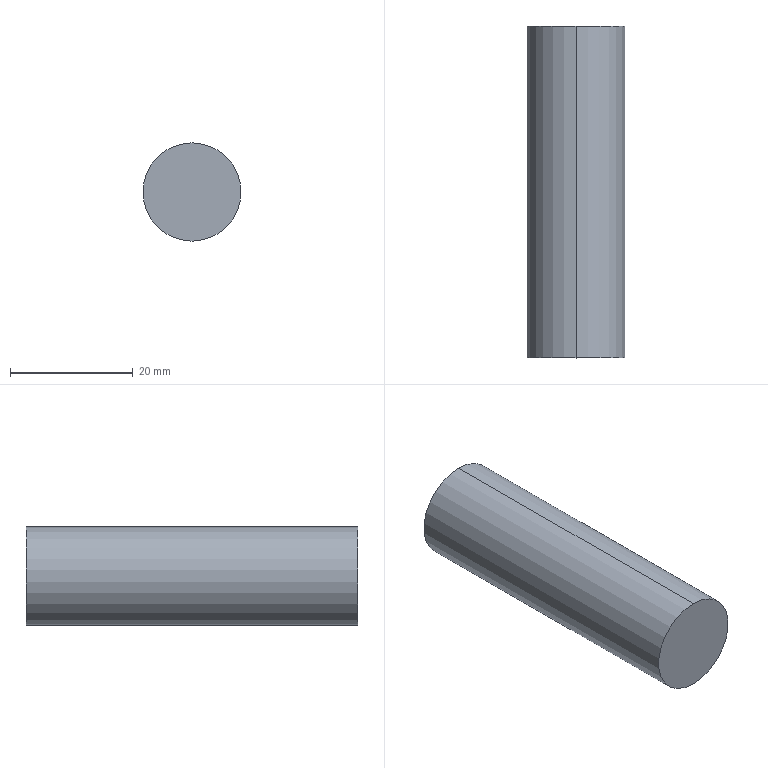Part | SolidWorks | features Extrusion 1 | 1 solid | 4 faces | box 16 x 54 x 16 mm | volume 10857 mm3 | cylinder 2 | plane 2 | commonest cylinder face diameters 16 x2
STEP:
#1=CARTESIAN_POINT('',(0.,54.,8.));
#2=VERTEX_POINT('',#1);
#3=CARTESIAN_POINT('',(0.,54.,-8.));
#4=VERTEX_POINT('',#3);
#5=CARTESIAN_POINT('',(0.,54.,0.));
#6=DIRECTION('',(0.,1.,0.));
#7=DIRECTION('',(0.,0.,1.));
#8=AXIS2_PLACEMENT_3D('',#5,#6,#7);
#9=CIRCLE('',#8,8.);
#10=EDGE_CURVE('',#2,#4,#9,.T.);
#11=ORIENTED_EDGE('',*,*,#10,.F.);
#12=CARTESIAN_POINT('',(0.,0.,8.));
#13=VERTEX_POINT('',#12);
#14=CARTESIAN_POINT('',(0.,54.,8.));
#15=DIRECTION('',(0.,-1.,0.));
#16=VECTOR('',#15,1000.);
#17=LINE('',#14,#16);
#18=EDGE_CURVE('',#2,#13,#17,.T.);
#19=ORIENTED_EDGE('',*,*,#18,.T.);
#20=CARTESIAN_POINT('',(0.,0.,-8.));
#21=VERTEX_POINT('',#20);
#22=CARTESIAN_POINT('',(0.,0.,0.));
#23=DIRECTION('',(0.,1.,0.));
#24=DIRECTION('',(0.,0.,1.));
#25=AXIS2_PLACEMENT_3D('',#22,#23,#24);
#26=CIRCLE('',#25,8.);
#27=EDGE_CURVE('',#13,#21,#26,.T.);
#28=ORIENTED_EDGE('',*,*,#27,.T.);
#29=CARTESIAN_POINT('',(0.,54.,-8.));
#30=DIRECTION('',(0.,-1.,0.));
#31=VECTOR('',#30,1000.);
#32=LINE('',#29,#31);
#33=EDGE_CURVE('',#4,#21,#32,.T.);
#34=ORIENTED_EDGE('',*,*,#33,.F.);
#35=EDGE_LOOP('',(#11,#19,#28,#34));
#36=FACE_OUTER_BOUND('',#35,.T.);
#37=CARTESIAN_POINT('',(0.,54.,0.));
#38=DIRECTION('',(0.,-1.,0.));
#39=DIRECTION('',(0.,0.,-1.));
#40=AXIS2_PLACEMENT_3D('',#37,#38,#39);
#41=CYLINDRICAL_SURFACE('',#40,8.);
#42=ADVANCED_FACE('',(#36),#41,.T.);
#43=ORIENTED_EDGE('',*,*,#18,.F.);
#44=CARTESIAN_POINT('',(0.,54.,0.));
#45=DIRECTION('',(0.,1.,0.));
#46=DIRECTION('',(0.,0.,1.));
#47=AXIS2_PLACEMENT_3D('',#44,#45,#46);
#48=CIRCLE('',#47,8.);
#49=EDGE_CURVE('',#4,#2,#48,.T.);
#50=ORIENTED_EDGE('',*,*,#49,.F.);
#51=ORIENTED_EDGE('',*,*,#33,.T.);
#52=CARTESIAN_POINT('',(0.,0.,0.));
#53=DIRECTION('',(0.,1.,0.));
#54=DIRECTION('',(0.,0.,1.));
#55=AXIS2_PLACEMENT_3D('',#52,#53,#54);
#56=CIRCLE('',#55,8.);
#57=EDGE_CURVE('',#21,#13,#56,.T.);
#58=ORIENTED_EDGE('',*,*,#57,.T.);
#59=EDGE_LOOP('',(#43,#50,#51,#58));
#60=FACE_OUTER_BOUND('',#59,.T.);
#61=CARTESIAN_POINT('',(0.,54.,0.));
#62=DIRECTION('',(0.,-1.,0.));
#63=DIRECTION('',(0.,0.,-1.));
#64=AXIS2_PLACEMENT_3D('',#61,#62,#63);
#65=CYLINDRICAL_SURFACE('',#64,8.);
#66=ADVANCED_FACE('',(#60),#65,.T.);
#67=ORIENTED_EDGE('',*,*,#49,.T.);
#68=ORIENTED_EDGE('',*,*,#10,.T.);
#69=EDGE_LOOP('',(#67,#68));
#70=FACE_OUTER_BOUND('',#69,.T.);
#71=CARTESIAN_POINT('',(0.,54.,0.));
#72=DIRECTION('',(0.,1.,0.));
#73=DIRECTION('',(0.,0.,1.));
#74=AXIS2_PLACEMENT_3D('',#71,#72,#73);
#75=PLANE('',#74);
#76=ADVANCED_FACE('',(#70),#75,.T.);
#77=ORIENTED_EDGE('',*,*,#57,.F.);
#78=ORIENTED_EDGE('',*,*,#27,.F.);
#79=EDGE_LOOP('',(#77,#78));
#80=FACE_OUTER_BOUND('',#79,.T.);
#81=CARTESIAN_POINT('',(0.,0.,0.));
#82=DIRECTION('',(0.,1.,0.));
#83=DIRECTION('',(0.,0.,1.));
#84=AXIS2_PLACEMENT_3D('',#81,#82,#83);
#85=PLANE('',#84);
#86=ADVANCED_FACE('',(#80),#85,.F.);
#87=CLOSED_SHELL('',(#42,#66,#76,#86));
#88=MANIFOLD_SOLID_BREP('',#87);
#89=CARTESIAN_POINT('',(0.,0.,0.));
#90=DIRECTION('',(0.,0.,1.));
#91=DIRECTION('',(1.,0.,0.));
#92=AXIS2_PLACEMENT_3D('',#89,#90,#91);
#93=(LENGTH_UNIT()NAMED_UNIT(*)SI_UNIT(.MILLI.,.METRE.));
#94=UNCERTAINTY_MEASURE_WITH_UNIT(LENGTH_MEASURE(0.00001),#93,'','');
#95=(NAMED_UNIT(*)PLANE_ANGLE_UNIT()SI_UNIT($,.RADIAN.));
#96=(NAMED_UNIT(*)SI_UNIT($,.STERADIAN.)SOLID_ANGLE_UNIT());
#97=(GEOMETRIC_REPRESENTATION_CONTEXT(3)GLOBAL_UNCERTAINTY_ASSIGNED_CONTEXT((#94))GLOBAL_UNIT_ASSIGNED_CONTEXT((#93,#95,#96))REPRESENTATION_CONTEXT('',''));
#98=ADVANCED_BREP_SHAPE_REPRESENTATION('',(#88,#92),#97);